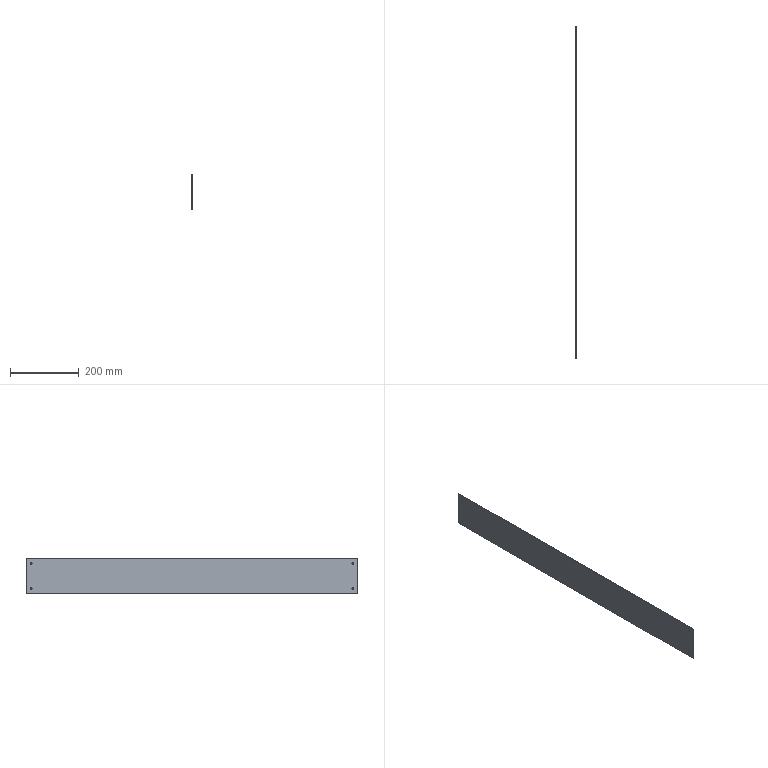Part | STEP file | PA-7-66(cover plate) | 1 solid | 14 faces | box 2 x 968 x 104 mm | volume 201187 mm3 | cylinder 8 | plane 6 | commonest cylinder face diameters 5 x8
STEP:
#1=CARTESIAN_POINT('',(0.,0.,0.));
#2=DIRECTION('',(0.,0.,1.));
#3=DIRECTION('',(1.,0.,0.));
#4=AXIS2_PLACEMENT_3D('',#1,#2,#3);
#5=CARTESIAN_POINT('',(-2.,469.,34.5));
#6=VERTEX_POINT('',#5);
#7=CARTESIAN_POINT('',(0.,469.,34.5));
#8=VERTEX_POINT('',#7);
#9=CARTESIAN_POINT('',(0.,469.,34.5));
#10=DIRECTION('',(1.,0.,0.));
#11=VECTOR('',#10,1.);
#12=LINE('',#9,#11);
#13=CARTESIAN_POINT('',(0.,469.,37.));
#14=DIRECTION('',(1.,0.,0.));
#15=DIRECTION('',(0.,0.,-1.));
#16=AXIS2_PLACEMENT_3D('',#13,#14,#15);
#17=CYLINDRICAL_SURFACE('',#16,2.5);
#18=CARTESIAN_POINT('',(6.283,0.));
#19=DIRECTION('',(0.,1.));
#20=VECTOR('',#19,1.);
#21=LINE('',#18,#20);
#22=(GEOMETRIC_REPRESENTATION_CONTEXT(2)PARAMETRIC_REPRESENTATION_CONTEXT()REPRESENTATION_CONTEXT('',''));
#23=DEFINITIONAL_REPRESENTATION('',(#21),#22);
#24=PCURVE('',#17,#23);
#25=CARTESIAN_POINT('',(0.,469.,37.));
#26=DIRECTION('',(1.,0.,0.));
#27=DIRECTION('',(0.,0.,-1.));
#28=AXIS2_PLACEMENT_3D('',#25,#26,#27);
#29=CYLINDRICAL_SURFACE('',#28,2.5);
#30=CARTESIAN_POINT('',(0.,0.));
#31=DIRECTION('',(0.,1.));
#32=VECTOR('',#31,1.);
#33=LINE('',#30,#32);
#34=(GEOMETRIC_REPRESENTATION_CONTEXT(2)PARAMETRIC_REPRESENTATION_CONTEXT()REPRESENTATION_CONTEXT('',''));
#35=DEFINITIONAL_REPRESENTATION('',(#33),#34);
#36=PCURVE('',#29,#35);
#37=SURFACE_CURVE('',#12,(#24,#36),.PCURVE_S1.);
#38=EDGE_CURVE('',#6,#8,#37,.T.);
#39=ORIENTED_EDGE('',*,*,#38,.T.);
#40=CARTESIAN_POINT('',(0.,469.,39.5));
#41=VERTEX_POINT('',#40);
#42=CARTESIAN_POINT('',(0.,469.,37.));
#43=DIRECTION('',(1.,0.,0.));
#44=DIRECTION('',(0.,0.,-1.));
#45=AXIS2_PLACEMENT_3D('',#42,#43,#44);
#46=CIRCLE('',#45,2.5);
#47=CARTESIAN_POINT('',(0.,0.));
#48=DIRECTION('',(1.,0.));
#49=VECTOR('',#48,1.);
#50=LINE('',#47,#49);
#51=(GEOMETRIC_REPRESENTATION_CONTEXT(2)PARAMETRIC_REPRESENTATION_CONTEXT()REPRESENTATION_CONTEXT('',''));
#52=DEFINITIONAL_REPRESENTATION('',(#50),#51);
#53=PCURVE('',#17,#52);
#54=CARTESIAN_POINT('',(0.,0.,0.));
#55=DIRECTION('',(1.,0.,0.));
#56=DIRECTION('',(0.,0.,-1.));
#57=AXIS2_PLACEMENT_3D('',#54,#55,#56);
#58=PLANE('',#57);
#59=CARTESIAN_POINT('',(-37.,469.));
#60=DIRECTION('',(1.,0.));
#61=AXIS2_PLACEMENT_2D('',#59,#60);
#62=CIRCLE('',#61,2.5);
#63=(GEOMETRIC_REPRESENTATION_CONTEXT(2)PARAMETRIC_REPRESENTATION_CONTEXT()REPRESENTATION_CONTEXT('',''));
#64=DEFINITIONAL_REPRESENTATION('',(#62),#63);
#65=PCURVE('',#58,#64);
#66=SURFACE_CURVE('',#46,(#53,#65),.PCURVE_S1.);
#67=EDGE_CURVE('',#41,#8,#66,.T.);
#68=ORIENTED_EDGE('',*,*,#67,.F.);
#69=CARTESIAN_POINT('',(-2.,469.,39.5));
#70=VERTEX_POINT('',#69);
#71=CARTESIAN_POINT('',(0.,469.,39.5));
#72=DIRECTION('',(1.,0.,0.));
#73=VECTOR('',#72,1.);
#74=LINE('',#71,#73);
#75=CARTESIAN_POINT('',(3.142,0.));
#76=DIRECTION('',(0.,1.));
#77=VECTOR('',#76,1.);
#78=LINE('',#75,#77);
#79=(GEOMETRIC_REPRESENTATION_CONTEXT(2)PARAMETRIC_REPRESENTATION_CONTEXT()REPRESENTATION_CONTEXT('',''));
#80=DEFINITIONAL_REPRESENTATION('',(#78),#79);
#81=PCURVE('',#17,#80);
#82=CARTESIAN_POINT('',(3.142,0.));
#83=DIRECTION('',(0.,1.));
#84=VECTOR('',#83,1.);
#85=LINE('',#82,#84);
#86=(GEOMETRIC_REPRESENTATION_CONTEXT(2)PARAMETRIC_REPRESENTATION_CONTEXT()REPRESENTATION_CONTEXT('',''));
#87=DEFINITIONAL_REPRESENTATION('',(#85),#86);
#88=PCURVE('',#29,#87);
#89=SURFACE_CURVE('',#74,(#81,#88),.PCURVE_S1.);
#90=EDGE_CURVE('',#70,#41,#89,.T.);
#91=ORIENTED_EDGE('',*,*,#90,.F.);
#92=CARTESIAN_POINT('',(-2.,469.,37.));
#93=DIRECTION('',(1.,0.,0.));
#94=DIRECTION('',(0.,0.,-1.));
#95=AXIS2_PLACEMENT_3D('',#92,#93,#94);
#96=CIRCLE('',#95,2.5);
#97=CARTESIAN_POINT('',(0.,-2.));
#98=DIRECTION('',(1.,0.));
#99=VECTOR('',#98,1.);
#100=LINE('',#97,#99);
#101=(GEOMETRIC_REPRESENTATION_CONTEXT(2)PARAMETRIC_REPRESENTATION_CONTEXT()REPRESENTATION_CONTEXT('',''));
#102=DEFINITIONAL_REPRESENTATION('',(#100),#101);
#103=PCURVE('',#17,#102);
#104=CARTESIAN_POINT('',(-2.,0.,0.));
#105=DIRECTION('',(1.,0.,0.));
#106=DIRECTION('',(0.,0.,-1.));
#107=AXIS2_PLACEMENT_3D('',#104,#105,#106);
#108=PLANE('',#107);
#109=CARTESIAN_POINT('',(-37.,469.));
#110=DIRECTION('',(1.,0.));
#111=AXIS2_PLACEMENT_2D('',#109,#110);
#112=CIRCLE('',#111,2.5);
#113=(GEOMETRIC_REPRESENTATION_CONTEXT(2)PARAMETRIC_REPRESENTATION_CONTEXT()REPRESENTATION_CONTEXT('',''));
#114=DEFINITIONAL_REPRESENTATION('',(#112),#113);
#115=PCURVE('',#108,#114);
#116=SURFACE_CURVE('',#96,(#103,#115),.PCURVE_S1.);
#117=EDGE_CURVE('',#70,#6,#116,.T.);
#118=ORIENTED_EDGE('',*,*,#117,.T.);
#119=EDGE_LOOP('',(#39,#68,#91,#118));
#120=FACE_BOUND('',#119,.F.);
#121=ADVANCED_FACE('',(#120),#17,.F.);
#122=CARTESIAN_POINT('',(-2.,-469.,34.5));
#123=VERTEX_POINT('',#122);
#124=CARTESIAN_POINT('',(0.,-469.,34.5));
#125=VERTEX_POINT('',#124);
#126=CARTESIAN_POINT('',(0.,-469.,34.5));
#127=DIRECTION('',(1.,0.,0.));
#128=VECTOR('',#127,1.);
#129=LINE('',#126,#128);
#130=CARTESIAN_POINT('',(0.,-469.,37.));
#131=DIRECTION('',(1.,0.,0.));
#132=DIRECTION('',(0.,0.,-1.));
#133=AXIS2_PLACEMENT_3D('',#130,#131,#132);
#134=CYLINDRICAL_SURFACE('',#133,2.5);
#135=CARTESIAN_POINT('',(6.283,0.));
#136=DIRECTION('',(0.,1.));
#137=VECTOR('',#136,1.);
#138=LINE('',#135,#137);
#139=(GEOMETRIC_REPRESENTATION_CONTEXT(2)PARAMETRIC_REPRESENTATION_CONTEXT()REPRESENTATION_CONTEXT('',''));
#140=DEFINITIONAL_REPRESENTATION('',(#138),#139);
#141=PCURVE('',#134,#140);
#142=CARTESIAN_POINT('',(0.,-469.,37.));
#143=DIRECTION('',(1.,0.,0.));
#144=DIRECTION('',(0.,0.,-1.));
#145=AXIS2_PLACEMENT_3D('',#142,#143,#144);
#146=CYLINDRICAL_SURFACE('',#145,2.5);
#147=CARTESIAN_POINT('',(0.,0.));
#148=DIRECTION('',(0.,1.));
#149=VECTOR('',#148,1.);
#150=LINE('',#147,#149);
#151=(GEOMETRIC_REPRESENTATION_CONTEXT(2)PARAMETRIC_REPRESENTATION_CONTEXT()REPRESENTATION_CONTEXT('',''));
#152=DEFINITIONAL_REPRESENTATION('',(#150),#151);
#153=PCURVE('',#146,#152);
#154=SURFACE_CURVE('',#129,(#141,#153),.PCURVE_S1.);
#155=EDGE_CURVE('',#123,#125,#154,.T.);
#156=ORIENTED_EDGE('',*,*,#155,.T.);
#157=CARTESIAN_POINT('',(0.,-469.,39.5));
#158=VERTEX_POINT('',#157);
#159=CARTESIAN_POINT('',(0.,-469.,37.));
#160=DIRECTION('',(1.,0.,0.));
#161=DIRECTION('',(0.,0.,-1.));
#162=AXIS2_PLACEMENT_3D('',#159,#160,#161);
#163=CIRCLE('',#162,2.5);
#164=CARTESIAN_POINT('',(0.,0.));
#165=DIRECTION('',(1.,0.));
#166=VECTOR('',#165,1.);
#167=LINE('',#164,#166);
#168=(GEOMETRIC_REPRESENTATION_CONTEXT(2)PARAMETRIC_REPRESENTATION_CONTEXT()REPRESENTATION_CONTEXT('',''));
#169=DEFINITIONAL_REPRESENTATION('',(#167),#168);
#170=PCURVE('',#134,#169);
#171=CARTESIAN_POINT('',(-37.,-469.));
#172=DIRECTION('',(1.,0.));
#173=AXIS2_PLACEMENT_2D('',#171,#172);
#174=CIRCLE('',#173,2.5);
#175=(GEOMETRIC_REPRESENTATION_CONTEXT(2)PARAMETRIC_REPRESENTATION_CONTEXT()REPRESENTATION_CONTEXT('',''));
#176=DEFINITIONAL_REPRESENTATION('',(#174),#175);
#177=PCURVE('',#58,#176);
#178=SURFACE_CURVE('',#163,(#170,#177),.PCURVE_S1.);
#179=EDGE_CURVE('',#158,#125,#178,.T.);
#180=ORIENTED_EDGE('',*,*,#179,.F.);
#181=CARTESIAN_POINT('',(-2.,-469.,39.5));
#182=VERTEX_POINT('',#181);
#183=CARTESIAN_POINT('',(0.,-469.,39.5));
#184=DIRECTION('',(1.,0.,0.));
#185=VECTOR('',#184,1.);
#186=LINE('',#183,#185);
#187=CARTESIAN_POINT('',(3.142,0.));
#188=DIRECTION('',(0.,1.));
#189=VECTOR('',#188,1.);
#190=LINE('',#187,#189);
#191=(GEOMETRIC_REPRESENTATION_CONTEXT(2)PARAMETRIC_REPRESENTATION_CONTEXT()REPRESENTATION_CONTEXT('',''));
#192=DEFINITIONAL_REPRESENTATION('',(#190),#191);
#193=PCURVE('',#134,#192);
#194=CARTESIAN_POINT('',(3.142,0.));
#195=DIRECTION('',(0.,1.));
#196=VECTOR('',#195,1.);
#197=LINE('',#194,#196);
#198=(GEOMETRIC_REPRESENTATION_CONTEXT(2)PARAMETRIC_REPRESENTATION_CONTEXT()REPRESENTATION_CONTEXT('',''));
#199=DEFINITIONAL_REPRESENTATION('',(#197),#198);
#200=PCURVE('',#146,#199);
#201=SURFACE_CURVE('',#186,(#193,#200),.PCURVE_S1.);
#202=EDGE_CURVE('',#182,#158,#201,.T.);
#203=ORIENTED_EDGE('',*,*,#202,.F.);
#204=CARTESIAN_POINT('',(-2.,-469.,37.));
#205=DIRECTION('',(1.,0.,0.));
#206=DIRECTION('',(0.,0.,-1.));
#207=AXIS2_PLACEMENT_3D('',#204,#205,#206);
#208=CIRCLE('',#207,2.5);
#209=CARTESIAN_POINT('',(0.,-2.));
#210=DIRECTION('',(1.,0.));
#211=VECTOR('',#210,1.);
#212=LINE('',#209,#211);
#213=(GEOMETRIC_REPRESENTATION_CONTEXT(2)PARAMETRIC_REPRESENTATION_CONTEXT()REPRESENTATION_CONTEXT('',''));
#214=DEFINITIONAL_REPRESENTATION('',(#212),#213);
#215=PCURVE('',#134,#214);
#216=CARTESIAN_POINT('',(-37.,-469.));
#217=DIRECTION('',(1.,0.));
#218=AXIS2_PLACEMENT_2D('',#216,#217);
#219=CIRCLE('',#218,2.5);
#220=(GEOMETRIC_REPRESENTATION_CONTEXT(2)PARAMETRIC_REPRESENTATION_CONTEXT()REPRESENTATION_CONTEXT('',''));
#221=DEFINITIONAL_REPRESENTATION('',(#219),#220);
#222=PCURVE('',#108,#221);
#223=SURFACE_CURVE('',#208,(#215,#222),.PCURVE_S1.);
#224=EDGE_CURVE('',#182,#123,#223,.T.);
#225=ORIENTED_EDGE('',*,*,#224,.T.);
#226=EDGE_LOOP('',(#156,#180,#203,#225));
#227=FACE_BOUND('',#226,.F.);
#228=ADVANCED_FACE('',(#227),#134,.F.);
#229=CARTESIAN_POINT('',(-2.,-469.,-39.5));
#230=VERTEX_POINT('',#229);
#231=CARTESIAN_POINT('',(0.,-469.,-39.5));
#232=VERTEX_POINT('',#231);
#233=CARTESIAN_POINT('',(0.,-469.,-39.5));
#234=DIRECTION('',(1.,0.,0.));
#235=VECTOR('',#234,1.);
#236=LINE('',#233,#235);
#237=CARTESIAN_POINT('',(0.,-469.,-37.));
#238=DIRECTION('',(1.,0.,0.));
#239=DIRECTION('',(0.,0.,-1.));
#240=AXIS2_PLACEMENT_3D('',#237,#238,#239);
#241=CYLINDRICAL_SURFACE('',#240,2.5);
#242=CARTESIAN_POINT('',(6.283,0.));
#243=DIRECTION('',(0.,1.));
#244=VECTOR('',#243,1.);
#245=LINE('',#242,#244);
#246=(GEOMETRIC_REPRESENTATION_CONTEXT(2)PARAMETRIC_REPRESENTATION_CONTEXT()REPRESENTATION_CONTEXT('',''));
#247=DEFINITIONAL_REPRESENTATION('',(#245),#246);
#248=PCURVE('',#241,#247);
#249=CARTESIAN_POINT('',(0.,-469.,-37.));
#250=DIRECTION('',(1.,0.,0.));
#251=DIRECTION('',(0.,0.,-1.));
#252=AXIS2_PLACEMENT_3D('',#249,#250,#251);
#253=CYLINDRICAL_SURFACE('',#252,2.5);
#254=CARTESIAN_POINT('',(0.,0.));
#255=DIRECTION('',(0.,1.));
#256=VECTOR('',#255,1.);
#257=LINE('',#254,#256);
#258=(GEOMETRIC_REPRESENTATION_CONTEXT(2)PARAMETRIC_REPRESENTATION_CONTEXT()REPRESENTATION_CONTEXT('',''));
#259=DEFINITIONAL_REPRESENTATION('',(#257),#258);
#260=PCURVE('',#253,#259);
#261=SURFACE_CURVE('',#236,(#248,#260),.PCURVE_S1.);
#262=EDGE_CURVE('',#230,#232,#261,.T.);
#263=ORIENTED_EDGE('',*,*,#262,.T.);
#264=CARTESIAN_POINT('',(0.,-469.,-34.5));
#265=VERTEX_POINT('',#264);
#266=CARTESIAN_POINT('',(0.,-469.,-37.));
#267=DIRECTION('',(1.,0.,0.));
#268=DIRECTION('',(0.,0.,-1.));
#269=AXIS2_PLACEMENT_3D('',#266,#267,#268);
#270=CIRCLE('',#269,2.5);
#271=CARTESIAN_POINT('',(0.,0.));
#272=DIRECTION('',(1.,0.));
#273=VECTOR('',#272,1.);
#274=LINE('',#271,#273);
#275=(GEOMETRIC_REPRESENTATION_CONTEXT(2)PARAMETRIC_REPRESENTATION_CONTEXT()REPRESENTATION_CONTEXT('',''));
#276=DEFINITIONAL_REPRESENTATION('',(#274),#275);
#277=PCURVE('',#241,#276);
#278=CARTESIAN_POINT('',(37.,-469.));
#279=DIRECTION('',(1.,0.));
#280=AXIS2_PLACEMENT_2D('',#278,#279);
#281=CIRCLE('',#280,2.5);
#282=(GEOMETRIC_REPRESENTATION_CONTEXT(2)PARAMETRIC_REPRESENTATION_CONTEXT()REPRESENTATION_CONTEXT('',''));
#283=DEFINITIONAL_REPRESENTATION('',(#281),#282);
#284=PCURVE('',#58,#283);
#285=SURFACE_CURVE('',#270,(#277,#284),.PCURVE_S1.);
#286=EDGE_CURVE('',#265,#232,#285,.T.);
#287=ORIENTED_EDGE('',*,*,#286,.F.);
#288=CARTESIAN_POINT('',(-2.,-469.,-34.5));
#289=VERTEX_POINT('',#288);
#290=CARTESIAN_POINT('',(0.,-469.,-34.5));
#291=DIRECTION('',(1.,0.,0.));
#292=VECTOR('',#291,1.);
#293=LINE('',#290,#292);
#294=CARTESIAN_POINT('',(3.142,0.));
#295=DIRECTION('',(0.,1.));
#296=VECTOR('',#295,1.);
#297=LINE('',#294,#296);
#298=(GEOMETRIC_REPRESENTATION_CONTEXT(2)PARAMETRIC_REPRESENTATION_CONTEXT()REPRESENTATION_CONTEXT('',''));
#299=DEFINITIONAL_REPRESENTATION('',(#297),#298);
#300=PCURVE('',#241,#299);
#301=CARTESIAN_POINT('',(3.142,0.));
#302=DIRECTION('',(0.,1.));
#303=VECTOR('',#302,1.);
#304=LINE('',#301,#303);
#305=(GEOMETRIC_REPRESENTATION_CONTEXT(2)PARAMETRIC_REPRESENTATION_CONTEXT()REPRESENTATION_CONTEXT('',''));
#306=DEFINITIONAL_REPRESENTATION('',(#304),#305);
#307=PCURVE('',#253,#306);
#308=SURFACE_CURVE('',#293,(#300,#307),.PCURVE_S1.);
#309=EDGE_CURVE('',#289,#265,#308,.T.);
#310=ORIENTED_EDGE('',*,*,#309,.F.);
#311=CARTESIAN_POINT('',(-2.,-469.,-37.));
#312=DIRECTION('',(1.,0.,0.));
#313=DIRECTION('',(0.,0.,-1.));
#314=AXIS2_PLACEMENT_3D('',#311,#312,#313);
#315=CIRCLE('',#314,2.5);
#316=CARTESIAN_POINT('',(0.,-2.));
#317=DIRECTION('',(1.,0.));
#318=VECTOR('',#317,1.);
#319=LINE('',#316,#318);
#320=(GEOMETRIC_REPRESENTATION_CONTEXT(2)PARAMETRIC_REPRESENTATION_CONTEXT()REPRESENTATION_CONTEXT('',''));
#321=DEFINITIONAL_REPRESENTATION('',(#319),#320);
#322=PCURVE('',#241,#321);
#323=CARTESIAN_POINT('',(37.,-469.));
#324=DIRECTION('',(1.,0.));
#325=AXIS2_PLACEMENT_2D('',#323,#324);
#326=CIRCLE('',#325,2.5);
#327=(GEOMETRIC_REPRESENTATION_CONTEXT(2)PARAMETRIC_REPRESENTATION_CONTEXT()REPRESENTATION_CONTEXT('',''));
#328=DEFINITIONAL_REPRESENTATION('',(#326),#327);
#329=PCURVE('',#108,#328);
#330=SURFACE_CURVE('',#315,(#322,#329),.PCURVE_S1.);
#331=EDGE_CURVE('',#289,#230,#330,.T.);
#332=ORIENTED_EDGE('',*,*,#331,.T.);
#333=EDGE_LOOP('',(#263,#287,#310,#332));
#334=FACE_BOUND('',#333,.F.);
#335=ADVANCED_FACE('',(#334),#241,.F.);
#336=CARTESIAN_POINT('',(-2.,469.,-39.5));
#337=VERTEX_POINT('',#336);
#338=CARTESIAN_POINT('',(0.,469.,-39.5));
#339=VERTEX_POINT('',#338);
#340=CARTESIAN_POINT('',(0.,469.,-39.5));
#341=DIRECTION('',(1.,0.,0.));
#342=VECTOR('',#341,1.);
#343=LINE('',#340,#342);
#344=CARTESIAN_POINT('',(0.,469.,-37.));
#345=DIRECTION('',(1.,0.,0.));
#346=DIRECTION('',(0.,0.,-1.));
#347=AXIS2_PLACEMENT_3D('',#344,#345,#346);
#348=CYLINDRICAL_SURFACE('',#347,2.5);
#349=CARTESIAN_POINT('',(6.283,0.));
#350=DIRECTION('',(0.,1.));
#351=VECTOR('',#350,1.);
#352=LINE('',#349,#351);
#353=(GEOMETRIC_REPRESENTATION_CONTEXT(2)PARAMETRIC_REPRESENTATION_CONTEXT()REPRESENTATION_CONTEXT('',''));
#354=DEFINITIONAL_REPRESENTATION('',(#352),#353);
#355=PCURVE('',#348,#354);
#356=CARTESIAN_POINT('',(0.,469.,-37.));
#357=DIRECTION('',(1.,0.,0.));
#358=DIRECTION('',(0.,0.,-1.));
#359=AXIS2_PLACEMENT_3D('',#356,#357,#358);
#360=CYLINDRICAL_SURFACE('',#359,2.5);
#361=CARTESIAN_POINT('',(0.,0.));
#362=DIRECTION('',(0.,1.));
#363=VECTOR('',#362,1.);
#364=LINE('',#361,#363);
#365=(GEOMETRIC_REPRESENTATION_CONTEXT(2)PARAMETRIC_REPRESENTATION_CONTEXT()REPRESENTATION_CONTEXT('',''));
#366=DEFINITIONAL_REPRESENTATION('',(#364),#365);
#367=PCURVE('',#360,#366);
#368=SURFACE_CURVE('',#343,(#355,#367),.PCURVE_S1.);
#369=EDGE_CURVE('',#337,#339,#368,.T.);
#370=ORIENTED_EDGE('',*,*,#369,.T.);
#371=CARTESIAN_POINT('',(0.,469.,-34.5));
#372=VERTEX_POINT('',#371);
#373=CARTESIAN_POINT('',(0.,469.,-37.));
#374=DIRECTION('',(1.,0.,0.));
#375=DIRECTION('',(0.,0.,-1.));
#376=AXIS2_PLACEMENT_3D('',#373,#374,#375);
#377=CIRCLE('',#376,2.5);
#378=CARTESIAN_POINT('',(0.,0.));
#379=DIRECTION('',(1.,0.));
#380=VECTOR('',#379,1.);
#381=LINE('',#378,#380);
#382=(GEOMETRIC_REPRESENTATION_CONTEXT(2)PARAMETRIC_REPRESENTATION_CONTEXT()REPRESENTATION_CONTEXT('',''));
#383=DEFINITIONAL_REPRESENTATION('',(#381),#382);
#384=PCURVE('',#348,#383);
#385=CARTESIAN_POINT('',(37.,469.));
#386=DIRECTION('',(1.,0.));
#387=AXIS2_PLACEMENT_2D('',#385,#386);
#388=CIRCLE('',#387,2.5);
#389=(GEOMETRIC_REPRESENTATION_CONTEXT(2)PARAMETRIC_REPRESENTATION_CONTEXT()REPRESENTATION_CONTEXT('',''));
#390=DEFINITIONAL_REPRESENTATION('',(#388),#389);
#391=PCURVE('',#58,#390);
#392=SURFACE_CURVE('',#377,(#384,#391),.PCURVE_S1.);
#393=EDGE_CURVE('',#372,#339,#392,.T.);
#394=ORIENTED_EDGE('',*,*,#393,.F.);
#395=CARTESIAN_POINT('',(-2.,469.,-34.5));
#396=VERTEX_POINT('',#395);
#397=CARTESIAN_POINT('',(0.,469.,-34.5));
#398=DIRECTION('',(1.,0.,0.));
#399=VECTOR('',#398,1.);
#400=LINE('',#397,#399);
#401=CARTESIAN_POINT('',(3.142,0.));
#402=DIRECTION('',(0.,1.));
#403=VECTOR('',#402,1.);
#404=LINE('',#401,#403);
#405=(GEOMETRIC_REPRESENTATION_CONTEXT(2)PARAMETRIC_REPRESENTATION_CONTEXT()REPRESENTATION_CONTEXT('',''));
#406=DEFINITIONAL_REPRESENTATION('',(#404),#405);
#407=PCURVE('',#348,#406);
#408=CARTESIAN_POINT('',(3.142,0.));
#409=DIRECTION('',(0.,1.));
#410=VECTOR('',#409,1.);
#411=LINE('',#408,#410);
#412=(GEOMETRIC_REPRESENTATION_CONTEXT(2)PARAMETRIC_REPRESENTATION_CONTEXT()REPRESENTATION_CONTEXT('',''));
#413=DEFINITIONAL_REPRESENTATION('',(#411),#412);
#414=PCURVE('',#360,#413);
#415=SURFACE_CURVE('',#400,(#407,#414),.PCURVE_S1.);
#416=EDGE_CURVE('',#396,#372,#415,.T.);
#417=ORIENTED_EDGE('',*,*,#416,.F.);
#418=CARTESIAN_POINT('',(-2.,469.,-37.));
#419=DIRECTION('',(1.,0.,0.));
#420=DIRECTION('',(0.,0.,-1.));
#421=AXIS2_PLACEMENT_3D('',#418,#419,#420);
#422=CIRCLE('',#421,2.5);
#423=CARTESIAN_POINT('',(0.,-2.));
#424=DIRECTION('',(1.,0.));
#425=VECTOR('',#424,1.);
#426=LINE('',#423,#425);
#427=(GEOMETRIC_REPRESENTATION_CONTEXT(2)PARAMETRIC_REPRESENTATION_CONTEXT()REPRESENTATION_CONTEXT('',''));
#428=DEFINITIONAL_REPRESENTATION('',(#426),#427);
#429=PCURVE('',#348,#428);
#430=CARTESIAN_POINT('',(37.,469.));
#431=DIRECTION('',(1.,0.));
#432=AXIS2_PLACEMENT_2D('',#430,#431);
#433=CIRCLE('',#432,2.5);
#434=(GEOMETRIC_REPRESENTATION_CONTEXT(2)PARAMETRIC_REPRESENTATION_CONTEXT()REPRESENTATION_CONTEXT('',''));
#435=DEFINITIONAL_REPRESENTATION('',(#433),#434);
#436=PCURVE('',#108,#435);
#437=SURFACE_CURVE('',#422,(#429,#436),.PCURVE_S1.);
#438=EDGE_CURVE('',#396,#337,#437,.T.);
#439=ORIENTED_EDGE('',*,*,#438,.T.);
#440=EDGE_LOOP('',(#370,#394,#417,#439));
#441=FACE_BOUND('',#440,.F.);
#442=ADVANCED_FACE('',(#441),#348,.F.);
#443=CARTESIAN_POINT('',(0.,484.,52.));
#444=VERTEX_POINT('',#443);
#445=CARTESIAN_POINT('',(0.,-484.,52.));
#446=VERTEX_POINT('',#445);
#447=CARTESIAN_POINT('',(0.,-484.,52.));
#448=DIRECTION('',(0.,-1.,0.));
#449=VECTOR('',#448,1.);
#450=LINE('',#447,#449);
#451=CARTESIAN_POINT('',(-2.,-484.,52.));
#452=DIRECTION('',(0.,0.,1.));
#453=DIRECTION('',(1.,0.,0.));
#454=AXIS2_PLACEMENT_3D('',#451,#452,#453);
#455=PLANE('',#454);
#456=CARTESIAN_POINT('',(2.,0.));
#457=DIRECTION('',(0.,-1.));
#458=VECTOR('',#457,1.);
#459=LINE('',#456,#458);
#460=(GEOMETRIC_REPRESENTATION_CONTEXT(2)PARAMETRIC_REPRESENTATION_CONTEXT()REPRESENTATION_CONTEXT('',''));
#461=DEFINITIONAL_REPRESENTATION('',(#459),#460);
#462=PCURVE('',#455,#461);
#463=CARTESIAN_POINT('',(-52.,-484.));
#464=DIRECTION('',(0.,-1.));
#465=VECTOR('',#464,1.);
#466=LINE('',#463,#465);
#467=(GEOMETRIC_REPRESENTATION_CONTEXT(2)PARAMETRIC_REPRESENTATION_CONTEXT()REPRESENTATION_CONTEXT('',''));
#468=DEFINITIONAL_REPRESENTATION('',(#466),#467);
#469=PCURVE('',#58,#468);
#470=SURFACE_CURVE('',#450,(#462,#469),.PCURVE_S1.);
#471=EDGE_CURVE('',#444,#446,#470,.T.);
#472=ORIENTED_EDGE('',*,*,#471,.F.);
#473=CARTESIAN_POINT('',(-2.,484.,52.));
#474=VERTEX_POINT('',#473);
#475=CARTESIAN_POINT('',(-2.,484.,52.));
#476=DIRECTION('',(1.,0.,0.));
#477=VECTOR('',#476,1.);
#478=LINE('',#475,#477);
#479=CARTESIAN_POINT('',(0.,968.));
#480=DIRECTION('',(1.,0.));
#481=VECTOR('',#480,1.);
#482=LINE('',#479,#481);
#483=(GEOMETRIC_REPRESENTATION_CONTEXT(2)PARAMETRIC_REPRESENTATION_CONTEXT()REPRESENTATION_CONTEXT('',''));
#484=DEFINITIONAL_REPRESENTATION('',(#482),#483);
#485=PCURVE('',#455,#484);
#486=CARTESIAN_POINT('',(-2.,484.,-52.));
#487=DIRECTION('',(0.,1.,0.));
#488=DIRECTION('',(0.,0.,1.));
#489=AXIS2_PLACEMENT_3D('',#486,#487,#488);
#490=PLANE('',#489);
#491=CARTESIAN_POINT('',(104.,0.));
#492=DIRECTION('',(0.,1.));
#493=VECTOR('',#492,1.);
#494=LINE('',#491,#493);
#495=(GEOMETRIC_REPRESENTATION_CONTEXT(2)PARAMETRIC_REPRESENTATION_CONTEXT()REPRESENTATION_CONTEXT('',''));
#496=DEFINITIONAL_REPRESENTATION('',(#494),#495);
#497=PCURVE('',#490,#496);
#498=SURFACE_CURVE('',#478,(#485,#497),.PCURVE_S1.);
#499=EDGE_CURVE('',#474,#444,#498,.T.);
#500=ORIENTED_EDGE('',*,*,#499,.F.);
#501=CARTESIAN_POINT('',(-2.,-484.,52.));
#502=VERTEX_POINT('',#501);
#503=CARTESIAN_POINT('',(-2.,-484.,52.));
#504=DIRECTION('',(0.,-1.,0.));
#505=VECTOR('',#504,1.);
#506=LINE('',#503,#505);
#507=CARTESIAN_POINT('',(0.,0.));
#508=DIRECTION('',(0.,-1.));
#509=VECTOR('',#508,1.);
#510=LINE('',#507,#509);
#511=(GEOMETRIC_REPRESENTATION_CONTEXT(2)PARAMETRIC_REPRESENTATION_CONTEXT()REPRESENTATION_CONTEXT('',''));
#512=DEFINITIONAL_REPRESENTATION('',(#510),#511);
#513=PCURVE('',#455,#512);
#514=CARTESIAN_POINT('',(-52.,-484.));
#515=DIRECTION('',(0.,-1.));
#516=VECTOR('',#515,1.);
#517=LINE('',#514,#516);
#518=(GEOMETRIC_REPRESENTATION_CONTEXT(2)PARAMETRIC_REPRESENTATION_CONTEXT()REPRESENTATION_CONTEXT('',''));
#519=DEFINITIONAL_REPRESENTATION('',(#517),#518);
#520=PCURVE('',#108,#519);
#521=SURFACE_CURVE('',#506,(#513,#520),.PCURVE_S1.);
#522=EDGE_CURVE('',#474,#502,#521,.T.);
#523=ORIENTED_EDGE('',*,*,#522,.T.);
#524=CARTESIAN_POINT('',(-2.,-484.,52.));
#525=DIRECTION('',(1.,0.,0.));
#526=VECTOR('',#525,1.);
#527=LINE('',#524,#526);
#528=CARTESIAN_POINT('',(0.,0.));
#529=DIRECTION('',(1.,0.));
#530=VECTOR('',#529,1.);
#531=LINE('',#528,#530);
#532=(GEOMETRIC_REPRESENTATION_CONTEXT(2)PARAMETRIC_REPRESENTATION_CONTEXT()REPRESENTATION_CONTEXT('',''));
#533=DEFINITIONAL_REPRESENTATION('',(#531),#532);
#534=PCURVE('',#455,#533);
#535=CARTESIAN_POINT('',(-2.,-484.,-52.));
#536=DIRECTION('',(0.,-1.,0.));
#537=DIRECTION('',(0.,0.,-1.));
#538=AXIS2_PLACEMENT_3D('',#535,#536,#537);
#539=PLANE('',#538);
#540=CARTESIAN_POINT('',(-104.,0.));
#541=DIRECTION('',(0.,1.));
#542=VECTOR('',#541,1.);
#543=LINE('',#540,#542);
#544=(GEOMETRIC_REPRESENTATION_CONTEXT(2)PARAMETRIC_REPRESENTATION_CONTEXT()REPRESENTATION_CONTEXT('',''));
#545=DEFINITIONAL_REPRESENTATION('',(#543),#544);
#546=PCURVE('',#539,#545);
#547=SURFACE_CURVE('',#527,(#534,#546),.PCURVE_S1.);
#548=EDGE_CURVE('',#502,#446,#547,.T.);
#549=ORIENTED_EDGE('',*,*,#548,.T.);
#550=EDGE_LOOP('',(#472,#500,#523,#549));
#551=FACE_BOUND('',#550,.T.);
#552=ADVANCED_FACE('',(#551),#455,.T.);
#553=CARTESIAN_POINT('',(0.,484.,-52.));
#554=VERTEX_POINT('',#553);
#555=CARTESIAN_POINT('',(0.,484.,-52.));
#556=DIRECTION('',(0.,0.,1.));
#557=VECTOR('',#556,1.);
#558=LINE('',#555,#557);
#559=CARTESIAN_POINT('',(0.,2.));
#560=DIRECTION('',(1.,0.));
#561=VECTOR('',#560,1.);
#562=LINE('',#559,#561);
#563=(GEOMETRIC_REPRESENTATION_CONTEXT(2)PARAMETRIC_REPRESENTATION_CONTEXT()REPRESENTATION_CONTEXT('',''));
#564=DEFINITIONAL_REPRESENTATION('',(#562),#563);
#565=PCURVE('',#490,#564);
#566=CARTESIAN_POINT('',(52.,484.));
#567=DIRECTION('',(-1.,0.));
#568=VECTOR('',#567,1.);
#569=LINE('',#566,#568);
#570=(GEOMETRIC_REPRESENTATION_CONTEXT(2)PARAMETRIC_REPRESENTATION_CONTEXT()REPRESENTATION_CONTEXT('',''));
#571=DEFINITIONAL_REPRESENTATION('',(#569),#570);
#572=PCURVE('',#58,#571);
#573=SURFACE_CURVE('',#558,(#565,#572),.PCURVE_S1.);
#574=EDGE_CURVE('',#554,#444,#573,.T.);
#575=ORIENTED_EDGE('',*,*,#574,.F.);
#576=CARTESIAN_POINT('',(-2.,484.,-52.));
#577=VERTEX_POINT('',#576);
#578=CARTESIAN_POINT('',(-2.,484.,-52.));
#579=DIRECTION('',(1.,0.,0.));
#580=VECTOR('',#579,1.);
#581=LINE('',#578,#580);
#582=CARTESIAN_POINT('',(0.,0.));
#583=DIRECTION('',(0.,1.));
#584=VECTOR('',#583,1.);
#585=LINE('',#582,#584);
#586=(GEOMETRIC_REPRESENTATION_CONTEXT(2)PARAMETRIC_REPRESENTATION_CONTEXT()REPRESENTATION_CONTEXT('',''));
#587=DEFINITIONAL_REPRESENTATION('',(#585),#586);
#588=PCURVE('',#490,#587);
#589=CARTESIAN_POINT('',(-2.,-484.,-52.));
#590=DIRECTION('',(0.,0.,-1.));
#591=DIRECTION('',(-1.,0.,0.));
#592=AXIS2_PLACEMENT_3D('',#589,#590,#591);
#593=PLANE('',#592);
#594=CARTESIAN_POINT('',(0.,968.));
#595=DIRECTION('',(-1.,0.));
#596=VECTOR('',#595,1.);
#597=LINE('',#594,#596);
#598=(GEOMETRIC_REPRESENTATION_CONTEXT(2)PARAMETRIC_REPRESENTATION_CONTEXT()REPRESENTATION_CONTEXT('',''));
#599=DEFINITIONAL_REPRESENTATION('',(#597),#598);
#600=PCURVE('',#593,#599);
#601=SURFACE_CURVE('',#581,(#588,#600),.PCURVE_S1.);
#602=EDGE_CURVE('',#577,#554,#601,.T.);
#603=ORIENTED_EDGE('',*,*,#602,.F.);
#604=CARTESIAN_POINT('',(-2.,484.,-52.));
#605=DIRECTION('',(0.,0.,1.));
#606=VECTOR('',#605,1.);
#607=LINE('',#604,#606);
#608=CARTESIAN_POINT('',(0.,0.));
#609=DIRECTION('',(1.,0.));
#610=VECTOR('',#609,1.);
#611=LINE('',#608,#610);
#612=(GEOMETRIC_REPRESENTATION_CONTEXT(2)PARAMETRIC_REPRESENTATION_CONTEXT()REPRESENTATION_CONTEXT('',''));
#613=DEFINITIONAL_REPRESENTATION('',(#611),#612);
#614=PCURVE('',#490,#613);
#615=CARTESIAN_POINT('',(52.,484.));
#616=DIRECTION('',(-1.,0.));
#617=VECTOR('',#616,1.);
#618=LINE('',#615,#617);
#619=(GEOMETRIC_REPRESENTATION_CONTEXT(2)PARAMETRIC_REPRESENTATION_CONTEXT()REPRESENTATION_CONTEXT('',''));
#620=DEFINITIONAL_REPRESENTATION('',(#618),#619);
#621=PCURVE('',#108,#620);
#622=SURFACE_CURVE('',#607,(#614,#621),.PCURVE_S1.);
#623=EDGE_CURVE('',#577,#474,#622,.T.);
#624=ORIENTED_EDGE('',*,*,#623,.T.);
#625=ORIENTED_EDGE('',*,*,#499,.T.);
#626=EDGE_LOOP('',(#575,#603,#624,#625));
#627=FACE_BOUND('',#626,.T.);
#628=ADVANCED_FACE('',(#627),#490,.T.);
#629=CARTESIAN_POINT('',(0.,-484.,-52.));
#630=VERTEX_POINT('',#629);
#631=CARTESIAN_POINT('',(0.,-484.,-52.));
#632=DIRECTION('',(0.,1.,0.));
#633=VECTOR('',#632,1.);
#634=LINE('',#631,#633);
#635=CARTESIAN_POINT('',(-2.,0.));
#636=DIRECTION('',(0.,1.));
#637=VECTOR('',#636,1.);
#638=LINE('',#635,#637);
#639=(GEOMETRIC_REPRESENTATION_CONTEXT(2)PARAMETRIC_REPRESENTATION_CONTEXT()REPRESENTATION_CONTEXT('',''));
#640=DEFINITIONAL_REPRESENTATION('',(#638),#639);
#641=PCURVE('',#593,#640);
#642=CARTESIAN_POINT('',(52.,-484.));
#643=DIRECTION('',(0.,1.));
#644=VECTOR('',#643,1.);
#645=LINE('',#642,#644);
#646=(GEOMETRIC_REPRESENTATION_CONTEXT(2)PARAMETRIC_REPRESENTATION_CONTEXT()REPRESENTATION_CONTEXT('',''));
#647=DEFINITIONAL_REPRESENTATION('',(#645),#646);
#648=PCURVE('',#58,#647);
#649=SURFACE_CURVE('',#634,(#641,#648),.PCURVE_S1.);
#650=EDGE_CURVE('',#630,#554,#649,.T.);
#651=ORIENTED_EDGE('',*,*,#650,.F.);
#652=CARTESIAN_POINT('',(-2.,-484.,-52.));
#653=VERTEX_POINT('',#652);
#654=CARTESIAN_POINT('',(-2.,-484.,-52.));
#655=DIRECTION('',(1.,0.,0.));
#656=VECTOR('',#655,1.);
#657=LINE('',#654,#656);
#658=CARTESIAN_POINT('',(0.,0.));
#659=DIRECTION('',(-1.,0.));
#660=VECTOR('',#659,1.);
#661=LINE('',#658,#660);
#662=(GEOMETRIC_REPRESENTATION_CONTEXT(2)PARAMETRIC_REPRESENTATION_CONTEXT()REPRESENTATION_CONTEXT('',''));
#663=DEFINITIONAL_REPRESENTATION('',(#661),#662);
#664=PCURVE('',#593,#663);
#665=CARTESIAN_POINT('',(0.,0.));
#666=DIRECTION('',(0.,1.));
#667=VECTOR('',#666,1.);
#668=LINE('',#665,#667);
#669=(GEOMETRIC_REPRESENTATION_CONTEXT(2)PARAMETRIC_REPRESENTATION_CONTEXT()REPRESENTATION_CONTEXT('',''));
#670=DEFINITIONAL_REPRESENTATION('',(#668),#669);
#671=PCURVE('',#539,#670);
#672=SURFACE_CURVE('',#657,(#664,#671),.PCURVE_S1.);
#673=EDGE_CURVE('',#653,#630,#672,.T.);
#674=ORIENTED_EDGE('',*,*,#673,.F.);
#675=CARTESIAN_POINT('',(-2.,-484.,-52.));
#676=DIRECTION('',(0.,1.,0.));
#677=VECTOR('',#676,1.);
#678=LINE('',#675,#677);
#679=CARTESIAN_POINT('',(0.,0.));
#680=DIRECTION('',(0.,1.));
#681=VECTOR('',#680,1.);
#682=LINE('',#679,#681);
#683=(GEOMETRIC_REPRESENTATION_CONTEXT(2)PARAMETRIC_REPRESENTATION_CONTEXT()REPRESENTATION_CONTEXT('',''));
#684=DEFINITIONAL_REPRESENTATION('',(#682),#683);
#685=PCURVE('',#593,#684);
#686=CARTESIAN_POINT('',(52.,-484.));
#687=DIRECTION('',(0.,1.));
#688=VECTOR('',#687,1.);
#689=LINE('',#686,#688);
#690=(GEOMETRIC_REPRESENTATION_CONTEXT(2)PARAMETRIC_REPRESENTATION_CONTEXT()REPRESENTATION_CONTEXT('',''));
#691=DEFINITIONAL_REPRESENTATION('',(#689),#690);
#692=PCURVE('',#108,#691);
#693=SURFACE_CURVE('',#678,(#685,#692),.PCURVE_S1.);
#694=EDGE_CURVE('',#653,#577,#693,.T.);
#695=ORIENTED_EDGE('',*,*,#694,.T.);
#696=ORIENTED_EDGE('',*,*,#602,.T.);
#697=EDGE_LOOP('',(#651,#674,#695,#696));
#698=FACE_BOUND('',#697,.T.);
#699=ADVANCED_FACE('',(#698),#593,.T.);
#700=CARTESIAN_POINT('',(0.,-484.,-52.));
#701=DIRECTION('',(0.,0.,-1.));
#702=VECTOR('',#701,1.);
#703=LINE('',#700,#702);
#704=CARTESIAN_POINT('',(0.,2.));
#705=DIRECTION('',(1.,0.));
#706=VECTOR('',#705,1.);
#707=LINE('',#704,#706);
#708=(GEOMETRIC_REPRESENTATION_CONTEXT(2)PARAMETRIC_REPRESENTATION_CONTEXT()REPRESENTATION_CONTEXT('',''));
#709=DEFINITIONAL_REPRESENTATION('',(#707),#708);
#710=PCURVE('',#539,#709);
#711=CARTESIAN_POINT('',(52.,-484.));
#712=DIRECTION('',(1.,0.));
#713=VECTOR('',#712,1.);
#714=LINE('',#711,#713);
#715=(GEOMETRIC_REPRESENTATION_CONTEXT(2)PARAMETRIC_REPRESENTATION_CONTEXT()REPRESENTATION_CONTEXT('',''));
#716=DEFINITIONAL_REPRESENTATION('',(#714),#715);
#717=PCURVE('',#58,#716);
#718=SURFACE_CURVE('',#703,(#710,#717),.PCURVE_S1.);
#719=EDGE_CURVE('',#446,#630,#718,.T.);
#720=ORIENTED_EDGE('',*,*,#719,.F.);
#721=ORIENTED_EDGE('',*,*,#548,.F.);
#722=CARTESIAN_POINT('',(-2.,-484.,-52.));
#723=DIRECTION('',(0.,0.,-1.));
#724=VECTOR('',#723,1.);
#725=LINE('',#722,#724);
#726=CARTESIAN_POINT('',(0.,0.));
#727=DIRECTION('',(1.,0.));
#728=VECTOR('',#727,1.);
#729=LINE('',#726,#728);
#730=(GEOMETRIC_REPRESENTATION_CONTEXT(2)PARAMETRIC_REPRESENTATION_CONTEXT()REPRESENTATION_CONTEXT('',''));
#731=DEFINITIONAL_REPRESENTATION('',(#729),#730);
#732=PCURVE('',#539,#731);
#733=CARTESIAN_POINT('',(52.,-484.));
#734=DIRECTION('',(1.,0.));
#735=VECTOR('',#734,1.);
#736=LINE('',#733,#735);
#737=(GEOMETRIC_REPRESENTATION_CONTEXT(2)PARAMETRIC_REPRESENTATION_CONTEXT()REPRESENTATION_CONTEXT('',''));
#738=DEFINITIONAL_REPRESENTATION('',(#736),#737);
#739=PCURVE('',#108,#738);
#740=SURFACE_CURVE('',#725,(#732,#739),.PCURVE_S1.);
#741=EDGE_CURVE('',#502,#653,#740,.T.);
#742=ORIENTED_EDGE('',*,*,#741,.T.);
#743=ORIENTED_EDGE('',*,*,#673,.T.);
#744=EDGE_LOOP('',(#720,#721,#742,#743));
#745=FACE_BOUND('',#744,.T.);
#746=ADVANCED_FACE('',(#745),#539,.T.);
#747=CARTESIAN_POINT('',(-2.,469.,37.));
#748=DIRECTION('',(1.,0.,0.));
#749=DIRECTION('',(0.,0.,-1.));
#750=AXIS2_PLACEMENT_3D('',#747,#748,#749);
#751=CIRCLE('',#750,2.5);
#752=CARTESIAN_POINT('',(-37.,469.));
#753=DIRECTION('',(1.,0.));
#754=AXIS2_PLACEMENT_2D('',#752,#753);
#755=CIRCLE('',#754,2.5);
#756=(GEOMETRIC_REPRESENTATION_CONTEXT(2)PARAMETRIC_REPRESENTATION_CONTEXT()REPRESENTATION_CONTEXT('',''));
#757=DEFINITIONAL_REPRESENTATION('',(#755),#756);
#758=PCURVE('',#108,#757);
#759=CARTESIAN_POINT('',(0.,-2.));
#760=DIRECTION('',(1.,0.));
#761=VECTOR('',#760,1.);
#762=LINE('',#759,#761);
#763=(GEOMETRIC_REPRESENTATION_CONTEXT(2)PARAMETRIC_REPRESENTATION_CONTEXT()REPRESENTATION_CONTEXT('',''));
#764=DEFINITIONAL_REPRESENTATION('',(#762),#763);
#765=PCURVE('',#29,#764);
#766=SURFACE_CURVE('',#751,(#758,#765),.PCURVE_S1.);
#767=EDGE_CURVE('',#6,#70,#766,.T.);
#768=ORIENTED_EDGE('',*,*,#767,.T.);
#769=ORIENTED_EDGE('',*,*,#117,.T.);
#770=EDGE_LOOP('',(#768,#769));
#771=FACE_BOUND('',#770,.T.);
#772=CARTESIAN_POINT('',(-2.,-469.,37.));
#773=DIRECTION('',(1.,0.,0.));
#774=DIRECTION('',(0.,0.,-1.));
#775=AXIS2_PLACEMENT_3D('',#772,#773,#774);
#776=CIRCLE('',#775,2.5);
#777=CARTESIAN_POINT('',(-37.,-469.));
#778=DIRECTION('',(1.,0.));
#779=AXIS2_PLACEMENT_2D('',#777,#778);
#780=CIRCLE('',#779,2.5);
#781=(GEOMETRIC_REPRESENTATION_CONTEXT(2)PARAMETRIC_REPRESENTATION_CONTEXT()REPRESENTATION_CONTEXT('',''));
#782=DEFINITIONAL_REPRESENTATION('',(#780),#781);
#783=PCURVE('',#108,#782);
#784=CARTESIAN_POINT('',(0.,-2.));
#785=DIRECTION('',(1.,0.));
#786=VECTOR('',#785,1.);
#787=LINE('',#784,#786);
#788=(GEOMETRIC_REPRESENTATION_CONTEXT(2)PARAMETRIC_REPRESENTATION_CONTEXT()REPRESENTATION_CONTEXT('',''));
#789=DEFINITIONAL_REPRESENTATION('',(#787),#788);
#790=PCURVE('',#146,#789);
#791=SURFACE_CURVE('',#776,(#783,#790),.PCURVE_S1.);
#792=EDGE_CURVE('',#123,#182,#791,.T.);
#793=ORIENTED_EDGE('',*,*,#792,.T.);
#794=ORIENTED_EDGE('',*,*,#224,.T.);
#795=EDGE_LOOP('',(#793,#794));
#796=FACE_BOUND('',#795,.T.);
#797=CARTESIAN_POINT('',(-2.,-469.,-37.));
#798=DIRECTION('',(1.,0.,0.));
#799=DIRECTION('',(0.,0.,-1.));
#800=AXIS2_PLACEMENT_3D('',#797,#798,#799);
#801=CIRCLE('',#800,2.5);
#802=CARTESIAN_POINT('',(37.,-469.));
#803=DIRECTION('',(1.,0.));
#804=AXIS2_PLACEMENT_2D('',#802,#803);
#805=CIRCLE('',#804,2.5);
#806=(GEOMETRIC_REPRESENTATION_CONTEXT(2)PARAMETRIC_REPRESENTATION_CONTEXT()REPRESENTATION_CONTEXT('',''));
#807=DEFINITIONAL_REPRESENTATION('',(#805),#806);
#808=PCURVE('',#108,#807);
#809=CARTESIAN_POINT('',(0.,-2.));
#810=DIRECTION('',(1.,0.));
#811=VECTOR('',#810,1.);
#812=LINE('',#809,#811);
#813=(GEOMETRIC_REPRESENTATION_CONTEXT(2)PARAMETRIC_REPRESENTATION_CONTEXT()REPRESENTATION_CONTEXT('',''));
#814=DEFINITIONAL_REPRESENTATION('',(#812),#813);
#815=PCURVE('',#253,#814);
#816=SURFACE_CURVE('',#801,(#808,#815),.PCURVE_S1.);
#817=EDGE_CURVE('',#230,#289,#816,.T.);
#818=ORIENTED_EDGE('',*,*,#817,.T.);
#819=ORIENTED_EDGE('',*,*,#331,.T.);
#820=EDGE_LOOP('',(#818,#819));
#821=FACE_BOUND('',#820,.T.);
#822=CARTESIAN_POINT('',(-2.,469.,-37.));
#823=DIRECTION('',(1.,0.,0.));
#824=DIRECTION('',(0.,0.,-1.));
#825=AXIS2_PLACEMENT_3D('',#822,#823,#824);
#826=CIRCLE('',#825,2.5);
#827=CARTESIAN_POINT('',(37.,469.));
#828=DIRECTION('',(1.,0.));
#829=AXIS2_PLACEMENT_2D('',#827,#828);
#830=CIRCLE('',#829,2.5);
#831=(GEOMETRIC_REPRESENTATION_CONTEXT(2)PARAMETRIC_REPRESENTATION_CONTEXT()REPRESENTATION_CONTEXT('',''));
#832=DEFINITIONAL_REPRESENTATION('',(#830),#831);
#833=PCURVE('',#108,#832);
#834=CARTESIAN_POINT('',(0.,-2.));
#835=DIRECTION('',(1.,0.));
#836=VECTOR('',#835,1.);
#837=LINE('',#834,#836);
#838=(GEOMETRIC_REPRESENTATION_CONTEXT(2)PARAMETRIC_REPRESENTATION_CONTEXT()REPRESENTATION_CONTEXT('',''));
#839=DEFINITIONAL_REPRESENTATION('',(#837),#838);
#840=PCURVE('',#360,#839);
#841=SURFACE_CURVE('',#826,(#833,#840),.PCURVE_S1.);
#842=EDGE_CURVE('',#337,#396,#841,.T.);
#843=ORIENTED_EDGE('',*,*,#842,.T.);
#844=ORIENTED_EDGE('',*,*,#438,.T.);
#845=EDGE_LOOP('',(#843,#844));
#846=FACE_BOUND('',#845,.T.);
#847=ORIENTED_EDGE('',*,*,#522,.F.);
#848=ORIENTED_EDGE('',*,*,#623,.F.);
#849=ORIENTED_EDGE('',*,*,#694,.F.);
#850=ORIENTED_EDGE('',*,*,#741,.F.);
#851=EDGE_LOOP('',(#847,#848,#849,#850));
#852=FACE_BOUND('',#851,.T.);
#853=ADVANCED_FACE('',(#771,#796,#821,#846,#852),#108,.F.);
#854=CARTESIAN_POINT('',(0.,469.,37.));
#855=DIRECTION('',(1.,0.,0.));
#856=DIRECTION('',(0.,0.,-1.));
#857=AXIS2_PLACEMENT_3D('',#854,#855,#856);
#858=CIRCLE('',#857,2.5);
#859=CARTESIAN_POINT('',(-37.,469.));
#860=DIRECTION('',(1.,0.));
#861=AXIS2_PLACEMENT_2D('',#859,#860);
#862=CIRCLE('',#861,2.5);
#863=(GEOMETRIC_REPRESENTATION_CONTEXT(2)PARAMETRIC_REPRESENTATION_CONTEXT()REPRESENTATION_CONTEXT('',''));
#864=DEFINITIONAL_REPRESENTATION('',(#862),#863);
#865=PCURVE('',#58,#864);
#866=CARTESIAN_POINT('',(0.,0.));
#867=DIRECTION('',(1.,0.));
#868=VECTOR('',#867,1.);
#869=LINE('',#866,#868);
#870=(GEOMETRIC_REPRESENTATION_CONTEXT(2)PARAMETRIC_REPRESENTATION_CONTEXT()REPRESENTATION_CONTEXT('',''));
#871=DEFINITIONAL_REPRESENTATION('',(#869),#870);
#872=PCURVE('',#29,#871);
#873=SURFACE_CURVE('',#858,(#865,#872),.PCURVE_S1.);
#874=EDGE_CURVE('',#8,#41,#873,.T.);
#875=ORIENTED_EDGE('',*,*,#874,.F.);
#876=ORIENTED_EDGE('',*,*,#67,.F.);
#877=EDGE_LOOP('',(#875,#876));
#878=FACE_BOUND('',#877,.T.);
#879=CARTESIAN_POINT('',(0.,-469.,37.));
#880=DIRECTION('',(1.,0.,0.));
#881=DIRECTION('',(0.,0.,-1.));
#882=AXIS2_PLACEMENT_3D('',#879,#880,#881);
#883=CIRCLE('',#882,2.5);
#884=CARTESIAN_POINT('',(-37.,-469.));
#885=DIRECTION('',(1.,0.));
#886=AXIS2_PLACEMENT_2D('',#884,#885);
#887=CIRCLE('',#886,2.5);
#888=(GEOMETRIC_REPRESENTATION_CONTEXT(2)PARAMETRIC_REPRESENTATION_CONTEXT()REPRESENTATION_CONTEXT('',''));
#889=DEFINITIONAL_REPRESENTATION('',(#887),#888);
#890=PCURVE('',#58,#889);
#891=CARTESIAN_POINT('',(0.,0.));
#892=DIRECTION('',(1.,0.));
#893=VECTOR('',#892,1.);
#894=LINE('',#891,#893);
#895=(GEOMETRIC_REPRESENTATION_CONTEXT(2)PARAMETRIC_REPRESENTATION_CONTEXT()REPRESENTATION_CONTEXT('',''));
#896=DEFINITIONAL_REPRESENTATION('',(#894),#895);
#897=PCURVE('',#146,#896);
#898=SURFACE_CURVE('',#883,(#890,#897),.PCURVE_S1.);
#899=EDGE_CURVE('',#125,#158,#898,.T.);
#900=ORIENTED_EDGE('',*,*,#899,.F.);
#901=ORIENTED_EDGE('',*,*,#179,.F.);
#902=EDGE_LOOP('',(#900,#901));
#903=FACE_BOUND('',#902,.T.);
#904=CARTESIAN_POINT('',(0.,-469.,-37.));
#905=DIRECTION('',(1.,0.,0.));
#906=DIRECTION('',(0.,0.,-1.));
#907=AXIS2_PLACEMENT_3D('',#904,#905,#906);
#908=CIRCLE('',#907,2.5);
#909=CARTESIAN_POINT('',(37.,-469.));
#910=DIRECTION('',(1.,0.));
#911=AXIS2_PLACEMENT_2D('',#909,#910);
#912=CIRCLE('',#911,2.5);
#913=(GEOMETRIC_REPRESENTATION_CONTEXT(2)PARAMETRIC_REPRESENTATION_CONTEXT()REPRESENTATION_CONTEXT('',''));
#914=DEFINITIONAL_REPRESENTATION('',(#912),#913);
#915=PCURVE('',#58,#914);
#916=CARTESIAN_POINT('',(0.,0.));
#917=DIRECTION('',(1.,0.));
#918=VECTOR('',#917,1.);
#919=LINE('',#916,#918);
#920=(GEOMETRIC_REPRESENTATION_CONTEXT(2)PARAMETRIC_REPRESENTATION_CONTEXT()REPRESENTATION_CONTEXT('',''));
#921=DEFINITIONAL_REPRESENTATION('',(#919),#920);
#922=PCURVE('',#253,#921);
#923=SURFACE_CURVE('',#908,(#915,#922),.PCURVE_S1.);
#924=EDGE_CURVE('',#232,#265,#923,.T.);
#925=ORIENTED_EDGE('',*,*,#924,.F.);
#926=ORIENTED_EDGE('',*,*,#286,.F.);
#927=EDGE_LOOP('',(#925,#926));
#928=FACE_BOUND('',#927,.T.);
#929=CARTESIAN_POINT('',(0.,469.,-37.));
#930=DIRECTION('',(1.,0.,0.));
#931=DIRECTION('',(0.,0.,-1.));
#932=AXIS2_PLACEMENT_3D('',#929,#930,#931);
#933=CIRCLE('',#932,2.5);
#934=CARTESIAN_POINT('',(37.,469.));
#935=DIRECTION('',(1.,0.));
#936=AXIS2_PLACEMENT_2D('',#934,#935);
#937=CIRCLE('',#936,2.5);
#938=(GEOMETRIC_REPRESENTATION_CONTEXT(2)PARAMETRIC_REPRESENTATION_CONTEXT()REPRESENTATION_CONTEXT('',''));
#939=DEFINITIONAL_REPRESENTATION('',(#937),#938);
#940=PCURVE('',#58,#939);
#941=CARTESIAN_POINT('',(0.,0.));
#942=DIRECTION('',(1.,0.));
#943=VECTOR('',#942,1.);
#944=LINE('',#941,#943);
#945=(GEOMETRIC_REPRESENTATION_CONTEXT(2)PARAMETRIC_REPRESENTATION_CONTEXT()REPRESENTATION_CONTEXT('',''));
#946=DEFINITIONAL_REPRESENTATION('',(#944),#945);
#947=PCURVE('',#360,#946);
#948=SURFACE_CURVE('',#933,(#940,#947),.PCURVE_S1.);
#949=EDGE_CURVE('',#339,#372,#948,.T.);
#950=ORIENTED_EDGE('',*,*,#949,.F.);
#951=ORIENTED_EDGE('',*,*,#393,.F.);
#952=EDGE_LOOP('',(#950,#951));
#953=FACE_BOUND('',#952,.T.);
#954=ORIENTED_EDGE('',*,*,#471,.T.);
#955=ORIENTED_EDGE('',*,*,#719,.T.);
#956=ORIENTED_EDGE('',*,*,#650,.T.);
#957=ORIENTED_EDGE('',*,*,#574,.T.);
#958=EDGE_LOOP('',(#954,#955,#956,#957));
#959=FACE_BOUND('',#958,.T.);
#960=ADVANCED_FACE('',(#878,#903,#928,#953,#959),#58,.T.);
#961=ORIENTED_EDGE('',*,*,#949,.F.);
#962=ORIENTED_EDGE('',*,*,#369,.F.);
#963=ORIENTED_EDGE('',*,*,#842,.T.);
#964=ORIENTED_EDGE('',*,*,#416,.T.);
#965=EDGE_LOOP('',(#961,#962,#963,#964));
#966=FACE_BOUND('',#965,.F.);
#967=ADVANCED_FACE('',(#966),#360,.F.);
#968=ORIENTED_EDGE('',*,*,#924,.F.);
#969=ORIENTED_EDGE('',*,*,#262,.F.);
#970=ORIENTED_EDGE('',*,*,#817,.T.);
#971=ORIENTED_EDGE('',*,*,#309,.T.);
#972=EDGE_LOOP('',(#968,#969,#970,#971));
#973=FACE_BOUND('',#972,.F.);
#974=ADVANCED_FACE('',(#973),#253,.F.);
#975=ORIENTED_EDGE('',*,*,#899,.F.);
#976=ORIENTED_EDGE('',*,*,#155,.F.);
#977=ORIENTED_EDGE('',*,*,#792,.T.);
#978=ORIENTED_EDGE('',*,*,#202,.T.);
#979=EDGE_LOOP('',(#975,#976,#977,#978));
#980=FACE_BOUND('',#979,.F.);
#981=ADVANCED_FACE('',(#980),#146,.F.);
#982=ORIENTED_EDGE('',*,*,#874,.F.);
#983=ORIENTED_EDGE('',*,*,#38,.F.);
#984=ORIENTED_EDGE('',*,*,#767,.T.);
#985=ORIENTED_EDGE('',*,*,#90,.T.);
#986=EDGE_LOOP('',(#982,#983,#984,#985));
#987=FACE_BOUND('',#986,.F.);
#988=ADVANCED_FACE('',(#987),#29,.F.);
#989=CLOSED_SHELL('',(#121,#228,#335,#442,#552,#628,#699,#746,#853,#960,#967,#974,#981,#988));
#990=MANIFOLD_SOLID_BREP('',#989);
#991=(LENGTH_UNIT()NAMED_UNIT(*)SI_UNIT(.MILLI.,.METRE.));
#992=UNCERTAINTY_MEASURE_WITH_UNIT(LENGTH_MEASURE(0.0000001),#991,'','');
#993=(NAMED_UNIT(*)PLANE_ANGLE_UNIT()SI_UNIT($,.RADIAN.));
#994=(NAMED_UNIT(*)SI_UNIT($,.STERADIAN.)SOLID_ANGLE_UNIT());
#995=(GEOMETRIC_REPRESENTATION_CONTEXT(3)GLOBAL_UNCERTAINTY_ASSIGNED_CONTEXT((#992))GLOBAL_UNIT_ASSIGNED_CONTEXT((#991,#993,#994))REPRESENTATION_CONTEXT('',''));
#996=ADVANCED_BREP_SHAPE_REPRESENTATION('',(#4,#990),#995);